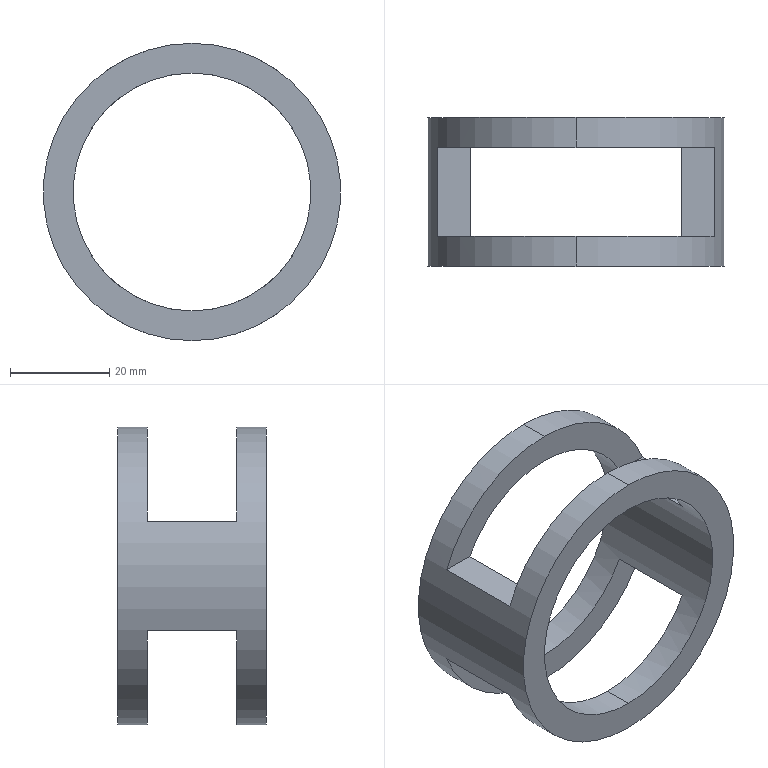Part | SolidWorks | features Extrusion 1, ICE 1 | 1 solid | 14 faces | box 60 x 30 x 60 mm | volume 17111 mm3 | plane 10 | cylinder 4 | commonest cylinder face diameters 48 x2 60 x2
STEP:
#1=CARTESIAN_POINT('',(0.,30.,-24.));
#2=VERTEX_POINT('',#1);
#3=CARTESIAN_POINT('',(0.,30.,24.));
#4=VERTEX_POINT('',#3);
#5=CARTESIAN_POINT('',(0.,30.,0.));
#6=DIRECTION('',(0.,1.,0.));
#7=DIRECTION('',(0.,0.,1.));
#8=AXIS2_PLACEMENT_3D('',#5,#6,#7);
#9=CIRCLE('',#8,24.);
#10=EDGE_CURVE('',#2,#4,#9,.T.);
#11=ORIENTED_EDGE('',*,*,#10,.T.);
#12=CARTESIAN_POINT('',(0.,24.,24.));
#13=VERTEX_POINT('',#12);
#14=CARTESIAN_POINT('',(0.,30.,24.));
#15=DIRECTION('',(0.,-1.,0.));
#16=VECTOR('',#15,1000.);
#17=LINE('',#14,#16);
#18=EDGE_CURVE('',#4,#13,#17,.T.);
#19=ORIENTED_EDGE('',*,*,#18,.T.);
#20=CARTESIAN_POINT('',(-21.331,24.,11.));
#21=VERTEX_POINT('',#20);
#22=CARTESIAN_POINT('',(0.,24.,0.));
#23=DIRECTION('',(0.,1.,0.));
#24=DIRECTION('',(0.,0.,1.));
#25=AXIS2_PLACEMENT_3D('',#22,#23,#24);
#26=CIRCLE('',#25,24.);
#27=EDGE_CURVE('',#21,#13,#26,.T.);
#28=ORIENTED_EDGE('',*,*,#27,.F.);
#29=CARTESIAN_POINT('',(-21.331,6.,11.));
#30=VERTEX_POINT('',#29);
#31=CARTESIAN_POINT('',(-21.331,30.,11.));
#32=DIRECTION('',(0.,1.,0.));
#33=VECTOR('',#32,1000.);
#34=LINE('',#31,#33);
#35=EDGE_CURVE('',#30,#21,#34,.T.);
#36=ORIENTED_EDGE('',*,*,#35,.F.);
#37=CARTESIAN_POINT('',(0.,6.,24.));
#38=VERTEX_POINT('',#37);
#39=CARTESIAN_POINT('',(0.,6.,0.));
#40=DIRECTION('',(0.,-1.,0.));
#41=DIRECTION('',(0.,0.,-1.));
#42=AXIS2_PLACEMENT_3D('',#39,#40,#41);
#43=CIRCLE('',#42,24.);
#44=EDGE_CURVE('',#38,#30,#43,.T.);
#45=ORIENTED_EDGE('',*,*,#44,.F.);
#46=CARTESIAN_POINT('',(0.,0.,24.));
#47=VERTEX_POINT('',#46);
#48=CARTESIAN_POINT('',(0.,30.,24.));
#49=DIRECTION('',(0.,-1.,0.));
#50=VECTOR('',#49,1000.);
#51=LINE('',#48,#50);
#52=EDGE_CURVE('',#38,#47,#51,.T.);
#53=ORIENTED_EDGE('',*,*,#52,.T.);
#54=CARTESIAN_POINT('',(0.,0.,-24.));
#55=VERTEX_POINT('',#54);
#56=CARTESIAN_POINT('',(0.,0.,0.));
#57=DIRECTION('',(0.,1.,0.));
#58=DIRECTION('',(0.,0.,1.));
#59=AXIS2_PLACEMENT_3D('',#56,#57,#58);
#60=CIRCLE('',#59,24.);
#61=EDGE_CURVE('',#55,#47,#60,.T.);
#62=ORIENTED_EDGE('',*,*,#61,.F.);
#63=CARTESIAN_POINT('',(0.,6.,-24.));
#64=VERTEX_POINT('',#63);
#65=CARTESIAN_POINT('',(0.,30.,-24.));
#66=DIRECTION('',(0.,-1.,0.));
#67=VECTOR('',#66,1000.);
#68=LINE('',#65,#67);
#69=EDGE_CURVE('',#64,#55,#68,.T.);
#70=ORIENTED_EDGE('',*,*,#69,.F.);
#71=CARTESIAN_POINT('',(-21.331,6.,-11.));
#72=VERTEX_POINT('',#71);
#73=CARTESIAN_POINT('',(0.,6.,0.));
#74=DIRECTION('',(0.,-1.,0.));
#75=DIRECTION('',(0.,0.,-1.));
#76=AXIS2_PLACEMENT_3D('',#73,#74,#75);
#77=CIRCLE('',#76,24.);
#78=EDGE_CURVE('',#72,#64,#77,.T.);
#79=ORIENTED_EDGE('',*,*,#78,.F.);
#80=CARTESIAN_POINT('',(-21.331,24.,-11.));
#81=VERTEX_POINT('',#80);
#82=CARTESIAN_POINT('',(-21.331,30.,-11.));
#83=DIRECTION('',(0.,-1.,0.));
#84=VECTOR('',#83,1000.);
#85=LINE('',#82,#84);
#86=EDGE_CURVE('',#81,#72,#85,.T.);
#87=ORIENTED_EDGE('',*,*,#86,.F.);
#88=CARTESIAN_POINT('',(0.,24.,-24.));
#89=VERTEX_POINT('',#88);
#90=CARTESIAN_POINT('',(0.,24.,0.));
#91=DIRECTION('',(0.,1.,0.));
#92=DIRECTION('',(0.,0.,1.));
#93=AXIS2_PLACEMENT_3D('',#90,#91,#92);
#94=CIRCLE('',#93,24.);
#95=EDGE_CURVE('',#89,#81,#94,.T.);
#96=ORIENTED_EDGE('',*,*,#95,.F.);
#97=CARTESIAN_POINT('',(0.,30.,-24.));
#98=DIRECTION('',(0.,-1.,0.));
#99=VECTOR('',#98,1000.);
#100=LINE('',#97,#99);
#101=EDGE_CURVE('',#2,#89,#100,.T.);
#102=ORIENTED_EDGE('',*,*,#101,.F.);
#103=EDGE_LOOP('',(#11,#19,#28,#36,#45,#53,#62,#70,#79,#87,#96,#102));
#104=FACE_OUTER_BOUND('',#103,.T.);
#105=CARTESIAN_POINT('',(0.,30.,0.));
#106=DIRECTION('',(0.,-1.,0.));
#107=DIRECTION('',(0.,0.,-1.));
#108=AXIS2_PLACEMENT_3D('',#105,#106,#107);
#109=CYLINDRICAL_SURFACE('',#108,24.);
#110=ADVANCED_FACE('',(#104),#109,.F.);
#111=CARTESIAN_POINT('',(0.,30.,30.));
#112=VERTEX_POINT('',#111);
#113=CARTESIAN_POINT('',(0.,30.,-30.));
#114=VERTEX_POINT('',#113);
#115=CARTESIAN_POINT('',(0.,30.,0.));
#116=DIRECTION('',(0.,1.,0.));
#117=DIRECTION('',(0.,0.,1.));
#118=AXIS2_PLACEMENT_3D('',#115,#116,#117);
#119=CIRCLE('',#118,30.);
#120=EDGE_CURVE('',#112,#114,#119,.T.);
#121=ORIENTED_EDGE('',*,*,#120,.F.);
#122=CARTESIAN_POINT('',(0.,24.,30.));
#123=VERTEX_POINT('',#122);
#124=CARTESIAN_POINT('',(0.,30.,30.));
#125=DIRECTION('',(0.,-1.,0.));
#126=VECTOR('',#125,1000.);
#127=LINE('',#124,#126);
#128=EDGE_CURVE('',#112,#123,#127,.T.);
#129=ORIENTED_EDGE('',*,*,#128,.T.);
#130=CARTESIAN_POINT('',(27.911,24.,11.));
#131=VERTEX_POINT('',#130);
#132=CARTESIAN_POINT('',(0.,24.,0.));
#133=DIRECTION('',(0.,1.,0.));
#134=DIRECTION('',(0.,0.,1.));
#135=AXIS2_PLACEMENT_3D('',#132,#133,#134);
#136=CIRCLE('',#135,30.);
#137=EDGE_CURVE('',#123,#131,#136,.T.);
#138=ORIENTED_EDGE('',*,*,#137,.T.);
#139=CARTESIAN_POINT('',(27.911,6.,11.));
#140=VERTEX_POINT('',#139);
#141=CARTESIAN_POINT('',(27.911,30.,11.));
#142=DIRECTION('',(0.,-1.,0.));
#143=VECTOR('',#142,1000.);
#144=LINE('',#141,#143);
#145=EDGE_CURVE('',#131,#140,#144,.T.);
#146=ORIENTED_EDGE('',*,*,#145,.T.);
#147=CARTESIAN_POINT('',(0.,6.,30.));
#148=VERTEX_POINT('',#147);
#149=CARTESIAN_POINT('',(0.,6.,0.));
#150=DIRECTION('',(0.,-1.,0.));
#151=DIRECTION('',(0.,0.,-1.));
#152=AXIS2_PLACEMENT_3D('',#149,#150,#151);
#153=CIRCLE('',#152,30.);
#154=EDGE_CURVE('',#140,#148,#153,.T.);
#155=ORIENTED_EDGE('',*,*,#154,.T.);
#156=CARTESIAN_POINT('',(0.,0.,30.));
#157=VERTEX_POINT('',#156);
#158=CARTESIAN_POINT('',(0.,30.,30.));
#159=DIRECTION('',(0.,-1.,0.));
#160=VECTOR('',#159,1000.);
#161=LINE('',#158,#160);
#162=EDGE_CURVE('',#148,#157,#161,.T.);
#163=ORIENTED_EDGE('',*,*,#162,.T.);
#164=CARTESIAN_POINT('',(0.,0.,-30.));
#165=VERTEX_POINT('',#164);
#166=CARTESIAN_POINT('',(0.,0.,0.));
#167=DIRECTION('',(0.,1.,0.));
#168=DIRECTION('',(0.,0.,1.));
#169=AXIS2_PLACEMENT_3D('',#166,#167,#168);
#170=CIRCLE('',#169,30.);
#171=EDGE_CURVE('',#157,#165,#170,.T.);
#172=ORIENTED_EDGE('',*,*,#171,.T.);
#173=CARTESIAN_POINT('',(0.,6.,-30.));
#174=VERTEX_POINT('',#173);
#175=CARTESIAN_POINT('',(0.,30.,-30.));
#176=DIRECTION('',(0.,-1.,0.));
#177=VECTOR('',#176,1000.);
#178=LINE('',#175,#177);
#179=EDGE_CURVE('',#174,#165,#178,.T.);
#180=ORIENTED_EDGE('',*,*,#179,.F.);
#181=CARTESIAN_POINT('',(27.911,6.,-11.));
#182=VERTEX_POINT('',#181);
#183=CARTESIAN_POINT('',(0.,6.,0.));
#184=DIRECTION('',(0.,-1.,0.));
#185=DIRECTION('',(0.,0.,-1.));
#186=AXIS2_PLACEMENT_3D('',#183,#184,#185);
#187=CIRCLE('',#186,30.);
#188=EDGE_CURVE('',#174,#182,#187,.T.);
#189=ORIENTED_EDGE('',*,*,#188,.T.);
#190=CARTESIAN_POINT('',(27.911,24.,-11.));
#191=VERTEX_POINT('',#190);
#192=CARTESIAN_POINT('',(27.911,30.,-11.));
#193=DIRECTION('',(0.,1.,0.));
#194=VECTOR('',#193,1000.);
#195=LINE('',#192,#194);
#196=EDGE_CURVE('',#182,#191,#195,.T.);
#197=ORIENTED_EDGE('',*,*,#196,.T.);
#198=CARTESIAN_POINT('',(0.,24.,-30.));
#199=VERTEX_POINT('',#198);
#200=CARTESIAN_POINT('',(0.,24.,0.));
#201=DIRECTION('',(0.,1.,0.));
#202=DIRECTION('',(0.,0.,1.));
#203=AXIS2_PLACEMENT_3D('',#200,#201,#202);
#204=CIRCLE('',#203,30.);
#205=EDGE_CURVE('',#191,#199,#204,.T.);
#206=ORIENTED_EDGE('',*,*,#205,.T.);
#207=CARTESIAN_POINT('',(0.,30.,-30.));
#208=DIRECTION('',(0.,-1.,0.));
#209=VECTOR('',#208,1000.);
#210=LINE('',#207,#209);
#211=EDGE_CURVE('',#114,#199,#210,.T.);
#212=ORIENTED_EDGE('',*,*,#211,.F.);
#213=EDGE_LOOP('',(#121,#129,#138,#146,#155,#163,#172,#180,#189,#197,#206,#212));
#214=FACE_OUTER_BOUND('',#213,.T.);
#215=CARTESIAN_POINT('',(0.,30.,0.));
#216=DIRECTION('',(0.,-1.,0.));
#217=DIRECTION('',(0.,0.,-1.));
#218=AXIS2_PLACEMENT_3D('',#215,#216,#217);
#219=CYLINDRICAL_SURFACE('',#218,30.);
#220=ADVANCED_FACE('',(#214),#219,.T.);
#221=CARTESIAN_POINT('',(0.,30.,0.));
#222=DIRECTION('',(0.,1.,0.));
#223=DIRECTION('',(0.,0.,1.));
#224=AXIS2_PLACEMENT_3D('',#221,#222,#223);
#225=CIRCLE('',#224,30.);
#226=EDGE_CURVE('',#114,#112,#225,.T.);
#227=ORIENTED_EDGE('',*,*,#226,.T.);
#228=ORIENTED_EDGE('',*,*,#120,.T.);
#229=EDGE_LOOP('',(#227,#228));
#230=FACE_OUTER_BOUND('',#229,.T.);
#231=ORIENTED_EDGE('',*,*,#10,.F.);
#232=CARTESIAN_POINT('',(0.,30.,0.));
#233=DIRECTION('',(0.,1.,0.));
#234=DIRECTION('',(0.,0.,1.));
#235=AXIS2_PLACEMENT_3D('',#232,#233,#234);
#236=CIRCLE('',#235,24.);
#237=EDGE_CURVE('',#4,#2,#236,.T.);
#238=ORIENTED_EDGE('',*,*,#237,.F.);
#239=EDGE_LOOP('',(#231,#238));
#240=FACE_BOUND('',#239,.T.);
#241=CARTESIAN_POINT('',(0.,30.,0.));
#242=DIRECTION('',(0.,1.,0.));
#243=DIRECTION('',(0.,0.,1.));
#244=AXIS2_PLACEMENT_3D('',#241,#242,#243);
#245=PLANE('',#244);
#246=ADVANCED_FACE('',(#230,#240),#245,.T.);
#247=CARTESIAN_POINT('',(0.,0.,0.));
#248=DIRECTION('',(0.,1.,0.));
#249=DIRECTION('',(0.,0.,1.));
#250=AXIS2_PLACEMENT_3D('',#247,#248,#249);
#251=CIRCLE('',#250,30.);
#252=EDGE_CURVE('',#165,#157,#251,.T.);
#253=ORIENTED_EDGE('',*,*,#252,.F.);
#254=ORIENTED_EDGE('',*,*,#171,.F.);
#255=EDGE_LOOP('',(#253,#254));
#256=FACE_OUTER_BOUND('',#255,.T.);
#257=ORIENTED_EDGE('',*,*,#61,.T.);
#258=CARTESIAN_POINT('',(0.,0.,0.));
#259=DIRECTION('',(0.,1.,0.));
#260=DIRECTION('',(0.,0.,1.));
#261=AXIS2_PLACEMENT_3D('',#258,#259,#260);
#262=CIRCLE('',#261,24.);
#263=EDGE_CURVE('',#47,#55,#262,.T.);
#264=ORIENTED_EDGE('',*,*,#263,.T.);
#265=EDGE_LOOP('',(#257,#264));
#266=FACE_BOUND('',#265,.T.);
#267=CARTESIAN_POINT('',(0.,0.,0.));
#268=DIRECTION('',(0.,1.,0.));
#269=DIRECTION('',(0.,0.,1.));
#270=AXIS2_PLACEMENT_3D('',#267,#268,#269);
#271=PLANE('',#270);
#272=ADVANCED_FACE('',(#256,#266),#271,.F.);
#273=ORIENTED_EDGE('',*,*,#128,.F.);
#274=ORIENTED_EDGE('',*,*,#226,.F.);
#275=ORIENTED_EDGE('',*,*,#211,.T.);
#276=CARTESIAN_POINT('',(-27.911,24.,-11.));
#277=VERTEX_POINT('',#276);
#278=CARTESIAN_POINT('',(0.,24.,0.));
#279=DIRECTION('',(0.,1.,0.));
#280=DIRECTION('',(0.,0.,1.));
#281=AXIS2_PLACEMENT_3D('',#278,#279,#280);
#282=CIRCLE('',#281,30.);
#283=EDGE_CURVE('',#199,#277,#282,.T.);
#284=ORIENTED_EDGE('',*,*,#283,.T.);
#285=CARTESIAN_POINT('',(-27.911,6.,-11.));
#286=VERTEX_POINT('',#285);
#287=CARTESIAN_POINT('',(-27.911,30.,-11.));
#288=DIRECTION('',(0.,-1.,0.));
#289=VECTOR('',#288,1000.);
#290=LINE('',#287,#289);
#291=EDGE_CURVE('',#277,#286,#290,.T.);
#292=ORIENTED_EDGE('',*,*,#291,.T.);
#293=CARTESIAN_POINT('',(0.,6.,0.));
#294=DIRECTION('',(0.,-1.,0.));
#295=DIRECTION('',(0.,0.,-1.));
#296=AXIS2_PLACEMENT_3D('',#293,#294,#295);
#297=CIRCLE('',#296,30.);
#298=EDGE_CURVE('',#286,#174,#297,.T.);
#299=ORIENTED_EDGE('',*,*,#298,.T.);
#300=ORIENTED_EDGE('',*,*,#179,.T.);
#301=ORIENTED_EDGE('',*,*,#252,.T.);
#302=ORIENTED_EDGE('',*,*,#162,.F.);
#303=CARTESIAN_POINT('',(-27.911,6.,11.));
#304=VERTEX_POINT('',#303);
#305=CARTESIAN_POINT('',(0.,6.,0.));
#306=DIRECTION('',(0.,-1.,0.));
#307=DIRECTION('',(0.,0.,-1.));
#308=AXIS2_PLACEMENT_3D('',#305,#306,#307);
#309=CIRCLE('',#308,30.);
#310=EDGE_CURVE('',#148,#304,#309,.T.);
#311=ORIENTED_EDGE('',*,*,#310,.T.);
#312=CARTESIAN_POINT('',(-27.911,24.,11.));
#313=VERTEX_POINT('',#312);
#314=CARTESIAN_POINT('',(-27.911,30.,11.));
#315=DIRECTION('',(0.,1.,0.));
#316=VECTOR('',#315,1000.);
#317=LINE('',#314,#316);
#318=EDGE_CURVE('',#304,#313,#317,.T.);
#319=ORIENTED_EDGE('',*,*,#318,.T.);
#320=CARTESIAN_POINT('',(0.,24.,0.));
#321=DIRECTION('',(0.,1.,0.));
#322=DIRECTION('',(0.,0.,1.));
#323=AXIS2_PLACEMENT_3D('',#320,#321,#322);
#324=CIRCLE('',#323,30.);
#325=EDGE_CURVE('',#313,#123,#324,.T.);
#326=ORIENTED_EDGE('',*,*,#325,.T.);
#327=EDGE_LOOP('',(#273,#274,#275,#284,#292,#299,#300,#301,#302,#311,#319,#326));
#328=FACE_OUTER_BOUND('',#327,.T.);
#329=CARTESIAN_POINT('',(0.,30.,0.));
#330=DIRECTION('',(0.,-1.,0.));
#331=DIRECTION('',(0.,0.,-1.));
#332=AXIS2_PLACEMENT_3D('',#329,#330,#331);
#333=CYLINDRICAL_SURFACE('',#332,30.);
#334=ADVANCED_FACE('',(#328),#333,.T.);
#335=ORIENTED_EDGE('',*,*,#18,.F.);
#336=ORIENTED_EDGE('',*,*,#237,.T.);
#337=ORIENTED_EDGE('',*,*,#101,.T.);
#338=CARTESIAN_POINT('',(21.331,24.,-11.));
#339=VERTEX_POINT('',#338);
#340=CARTESIAN_POINT('',(0.,24.,0.));
#341=DIRECTION('',(0.,1.,0.));
#342=DIRECTION('',(0.,0.,1.));
#343=AXIS2_PLACEMENT_3D('',#340,#341,#342);
#344=CIRCLE('',#343,24.);
#345=EDGE_CURVE('',#339,#89,#344,.T.);
#346=ORIENTED_EDGE('',*,*,#345,.F.);
#347=CARTESIAN_POINT('',(21.331,6.,-11.));
#348=VERTEX_POINT('',#347);
#349=CARTESIAN_POINT('',(21.331,30.,-11.));
#350=DIRECTION('',(0.,1.,0.));
#351=VECTOR('',#350,1000.);
#352=LINE('',#349,#351);
#353=EDGE_CURVE('',#348,#339,#352,.T.);
#354=ORIENTED_EDGE('',*,*,#353,.F.);
#355=CARTESIAN_POINT('',(0.,6.,0.));
#356=DIRECTION('',(0.,-1.,0.));
#357=DIRECTION('',(0.,0.,-1.));
#358=AXIS2_PLACEMENT_3D('',#355,#356,#357);
#359=CIRCLE('',#358,24.);
#360=EDGE_CURVE('',#64,#348,#359,.T.);
#361=ORIENTED_EDGE('',*,*,#360,.F.);
#362=ORIENTED_EDGE('',*,*,#69,.T.);
#363=ORIENTED_EDGE('',*,*,#263,.F.);
#364=ORIENTED_EDGE('',*,*,#52,.F.);
#365=CARTESIAN_POINT('',(21.331,6.,11.));
#366=VERTEX_POINT('',#365);
#367=CARTESIAN_POINT('',(0.,6.,0.));
#368=DIRECTION('',(0.,-1.,0.));
#369=DIRECTION('',(0.,0.,-1.));
#370=AXIS2_PLACEMENT_3D('',#367,#368,#369);
#371=CIRCLE('',#370,24.);
#372=EDGE_CURVE('',#366,#38,#371,.T.);
#373=ORIENTED_EDGE('',*,*,#372,.F.);
#374=CARTESIAN_POINT('',(21.331,24.,11.));
#375=VERTEX_POINT('',#374);
#376=CARTESIAN_POINT('',(21.331,30.,11.));
#377=DIRECTION('',(0.,-1.,0.));
#378=VECTOR('',#377,1000.);
#379=LINE('',#376,#378);
#380=EDGE_CURVE('',#375,#366,#379,.T.);
#381=ORIENTED_EDGE('',*,*,#380,.F.);
#382=CARTESIAN_POINT('',(0.,24.,0.));
#383=DIRECTION('',(0.,1.,0.));
#384=DIRECTION('',(0.,0.,1.));
#385=AXIS2_PLACEMENT_3D('',#382,#383,#384);
#386=CIRCLE('',#385,24.);
#387=EDGE_CURVE('',#13,#375,#386,.T.);
#388=ORIENTED_EDGE('',*,*,#387,.F.);
#389=EDGE_LOOP('',(#335,#336,#337,#346,#354,#361,#362,#363,#364,#373,#381,#388));
#390=FACE_OUTER_BOUND('',#389,.T.);
#391=CARTESIAN_POINT('',(0.,30.,0.));
#392=DIRECTION('',(0.,-1.,0.));
#393=DIRECTION('',(0.,0.,-1.));
#394=AXIS2_PLACEMENT_3D('',#391,#392,#393);
#395=CYLINDRICAL_SURFACE('',#394,24.);
#396=ADVANCED_FACE('',(#390),#395,.F.);
#397=CARTESIAN_POINT('',(-30.,6.,-11.));
#398=DIRECTION('',(1.,0.,0.));
#399=VECTOR('',#398,1000.);
#400=LINE('',#397,#399);
#401=EDGE_CURVE('',#286,#72,#400,.T.);
#402=ORIENTED_EDGE('',*,*,#401,.T.);
#403=ORIENTED_EDGE('',*,*,#78,.T.);
#404=ORIENTED_EDGE('',*,*,#360,.T.);
#405=CARTESIAN_POINT('',(-30.,6.,-11.));
#406=DIRECTION('',(1.,0.,0.));
#407=VECTOR('',#406,1000.);
#408=LINE('',#405,#407);
#409=EDGE_CURVE('',#348,#182,#408,.T.);
#410=ORIENTED_EDGE('',*,*,#409,.T.);
#411=ORIENTED_EDGE('',*,*,#188,.F.);
#412=ORIENTED_EDGE('',*,*,#298,.F.);
#413=EDGE_LOOP('',(#402,#403,#404,#410,#411,#412));
#414=FACE_OUTER_BOUND('',#413,.T.);
#415=CARTESIAN_POINT('',(-30.,6.,-49.));
#416=DIRECTION('',(0.,-1.,0.));
#417=DIRECTION('',(0.,0.,-1.));
#418=AXIS2_PLACEMENT_3D('',#415,#416,#417);
#419=PLANE('',#418);
#420=ADVANCED_FACE('',(#414),#419,.F.);
#421=CARTESIAN_POINT('',(-30.,24.,-11.));
#422=DIRECTION('',(1.,0.,0.));
#423=VECTOR('',#422,1000.);
#424=LINE('',#421,#423);
#425=EDGE_CURVE('',#277,#81,#424,.T.);
#426=ORIENTED_EDGE('',*,*,#425,.T.);
#427=ORIENTED_EDGE('',*,*,#86,.T.);
#428=ORIENTED_EDGE('',*,*,#401,.F.);
#429=ORIENTED_EDGE('',*,*,#291,.F.);
#430=EDGE_LOOP('',(#426,#427,#428,#429));
#431=FACE_OUTER_BOUND('',#430,.T.);
#432=CARTESIAN_POINT('',(-30.,6.,-11.));
#433=DIRECTION('',(0.,0.,1.));
#434=DIRECTION('',(0.,-1.,0.));
#435=AXIS2_PLACEMENT_3D('',#432,#433,#434);
#436=PLANE('',#435);
#437=ADVANCED_FACE('',(#431),#436,.F.);
#438=ORIENTED_EDGE('',*,*,#409,.F.);
#439=ORIENTED_EDGE('',*,*,#353,.T.);
#440=CARTESIAN_POINT('',(-30.,24.,-11.));
#441=DIRECTION('',(1.,0.,0.));
#442=VECTOR('',#441,1000.);
#443=LINE('',#440,#442);
#444=EDGE_CURVE('',#339,#191,#443,.T.);
#445=ORIENTED_EDGE('',*,*,#444,.T.);
#446=ORIENTED_EDGE('',*,*,#196,.F.);
#447=EDGE_LOOP('',(#438,#439,#445,#446));
#448=FACE_OUTER_BOUND('',#447,.T.);
#449=CARTESIAN_POINT('',(-30.,6.,-11.));
#450=DIRECTION('',(0.,0.,1.));
#451=DIRECTION('',(0.,-1.,0.));
#452=AXIS2_PLACEMENT_3D('',#449,#450,#451);
#453=PLANE('',#452);
#454=ADVANCED_FACE('',(#448),#453,.F.);
#455=ORIENTED_EDGE('',*,*,#444,.F.);
#456=ORIENTED_EDGE('',*,*,#345,.T.);
#457=ORIENTED_EDGE('',*,*,#95,.T.);
#458=ORIENTED_EDGE('',*,*,#425,.F.);
#459=ORIENTED_EDGE('',*,*,#283,.F.);
#460=ORIENTED_EDGE('',*,*,#205,.F.);
#461=EDGE_LOOP('',(#455,#456,#457,#458,#459,#460));
#462=FACE_OUTER_BOUND('',#461,.T.);
#463=CARTESIAN_POINT('',(-30.,24.,-49.));
#464=DIRECTION('',(0.,1.,0.));
#465=DIRECTION('',(0.,0.,1.));
#466=AXIS2_PLACEMENT_3D('',#463,#464,#465);
#467=PLANE('',#466);
#468=ADVANCED_FACE('',(#462),#467,.F.);
#469=CARTESIAN_POINT('',(-30.,24.,11.));
#470=DIRECTION('',(1.,0.,0.));
#471=VECTOR('',#470,1000.);
#472=LINE('',#469,#471);
#473=EDGE_CURVE('',#375,#131,#472,.T.);
#474=ORIENTED_EDGE('',*,*,#473,.F.);
#475=ORIENTED_EDGE('',*,*,#380,.T.);
#476=CARTESIAN_POINT('',(-30.,6.,11.));
#477=DIRECTION('',(1.,0.,0.));
#478=VECTOR('',#477,1000.);
#479=LINE('',#476,#478);
#480=EDGE_CURVE('',#366,#140,#479,.T.);
#481=ORIENTED_EDGE('',*,*,#480,.T.);
#482=ORIENTED_EDGE('',*,*,#145,.F.);
#483=EDGE_LOOP('',(#474,#475,#481,#482));
#484=FACE_OUTER_BOUND('',#483,.T.);
#485=CARTESIAN_POINT('',(-30.,6.,11.));
#486=DIRECTION('',(0.,0.,-1.));
#487=DIRECTION('',(-1.,0.,0.));
#488=AXIS2_PLACEMENT_3D('',#485,#486,#487);
#489=PLANE('',#488);
#490=ADVANCED_FACE('',(#484),#489,.F.);
#491=CARTESIAN_POINT('',(-30.,6.,11.));
#492=DIRECTION('',(1.,0.,0.));
#493=VECTOR('',#492,1000.);
#494=LINE('',#491,#493);
#495=EDGE_CURVE('',#304,#30,#494,.T.);
#496=ORIENTED_EDGE('',*,*,#495,.T.);
#497=ORIENTED_EDGE('',*,*,#35,.T.);
#498=CARTESIAN_POINT('',(-30.,24.,11.));
#499=DIRECTION('',(1.,0.,0.));
#500=VECTOR('',#499,1000.);
#501=LINE('',#498,#500);
#502=EDGE_CURVE('',#313,#21,#501,.T.);
#503=ORIENTED_EDGE('',*,*,#502,.F.);
#504=ORIENTED_EDGE('',*,*,#318,.F.);
#505=EDGE_LOOP('',(#496,#497,#503,#504));
#506=FACE_OUTER_BOUND('',#505,.T.);
#507=CARTESIAN_POINT('',(-30.,6.,11.));
#508=DIRECTION('',(0.,0.,-1.));
#509=DIRECTION('',(-1.,0.,0.));
#510=AXIS2_PLACEMENT_3D('',#507,#508,#509);
#511=PLANE('',#510);
#512=ADVANCED_FACE('',(#506),#511,.F.);
#513=ORIENTED_EDGE('',*,*,#480,.F.);
#514=ORIENTED_EDGE('',*,*,#372,.T.);
#515=ORIENTED_EDGE('',*,*,#44,.T.);
#516=ORIENTED_EDGE('',*,*,#495,.F.);
#517=ORIENTED_EDGE('',*,*,#310,.F.);
#518=ORIENTED_EDGE('',*,*,#154,.F.);
#519=EDGE_LOOP('',(#513,#514,#515,#516,#517,#518));
#520=FACE_OUTER_BOUND('',#519,.T.);
#521=CARTESIAN_POINT('',(-30.,6.,49.));
#522=DIRECTION('',(0.,-1.,0.));
#523=DIRECTION('',(0.,0.,-1.));
#524=AXIS2_PLACEMENT_3D('',#521,#522,#523);
#525=PLANE('',#524);
#526=ADVANCED_FACE('',(#520),#525,.F.);
#527=ORIENTED_EDGE('',*,*,#502,.T.);
#528=ORIENTED_EDGE('',*,*,#27,.T.);
#529=ORIENTED_EDGE('',*,*,#387,.T.);
#530=ORIENTED_EDGE('',*,*,#473,.T.);
#531=ORIENTED_EDGE('',*,*,#137,.F.);
#532=ORIENTED_EDGE('',*,*,#325,.F.);
#533=EDGE_LOOP('',(#527,#528,#529,#530,#531,#532));
#534=FACE_OUTER_BOUND('',#533,.T.);
#535=CARTESIAN_POINT('',(-30.,24.,49.));
#536=DIRECTION('',(0.,1.,0.));
#537=DIRECTION('',(0.,0.,1.));
#538=AXIS2_PLACEMENT_3D('',#535,#536,#537);
#539=PLANE('',#538);
#540=ADVANCED_FACE('',(#534),#539,.F.);
#541=CLOSED_SHELL('',(#110,#220,#246,#272,#334,#396,#420,#437,#454,#468,#490,#512,#526,#540));
#542=MANIFOLD_SOLID_BREP('',#541);
#543=CARTESIAN_POINT('',(0.,0.,0.));
#544=DIRECTION('',(0.,0.,1.));
#545=DIRECTION('',(1.,0.,0.));
#546=AXIS2_PLACEMENT_3D('',#543,#544,#545);
#547=(LENGTH_UNIT()NAMED_UNIT(*)SI_UNIT(.MILLI.,.METRE.));
#548=UNCERTAINTY_MEASURE_WITH_UNIT(LENGTH_MEASURE(0.00001),#547,'','');
#549=(NAMED_UNIT(*)PLANE_ANGLE_UNIT()SI_UNIT($,.RADIAN.));
#550=(NAMED_UNIT(*)SI_UNIT($,.STERADIAN.)SOLID_ANGLE_UNIT());
#551=(GEOMETRIC_REPRESENTATION_CONTEXT(3)GLOBAL_UNCERTAINTY_ASSIGNED_CONTEXT((#548))GLOBAL_UNIT_ASSIGNED_CONTEXT((#547,#549,#550))REPRESENTATION_CONTEXT('',''));
#552=ADVANCED_BREP_SHAPE_REPRESENTATION('',(#542,#546),#551);